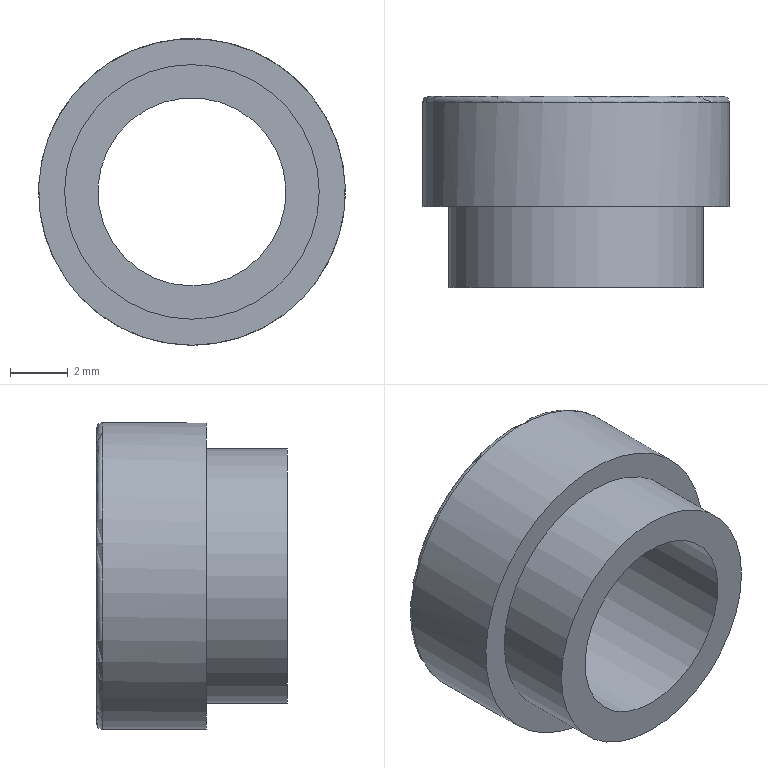Part | STEP file | 1 solid | 7 faces | box 10.6 x 6.6 x 10.6 mm | volume 286.348 mm3 | cylinder 3 | plane 3 | torus 1 | commonest cylinder face diameters 6.5 x1 8.8 x1 10.6 x1
STEP:
#1=CARTESIAN_POINT('',(0.,0.,0.));
#2=DIRECTION('',(0.,0.,1.));
#3=DIRECTION('',(1.,0.,0.));
#4=AXIS2_PLACEMENT_3D('',#1,#2,#3);
#5=CARTESIAN_POINT('',(0.,0.,-3.25));
#6=VERTEX_POINT('',#5);
#7=CARTESIAN_POINT('',(0.,0.,0.));
#8=DIRECTION('',(0.,1.,0.));
#9=DIRECTION('',(0.,0.,-1.));
#10=AXIS2_PLACEMENT_3D('',#7,#8,#9);
#11=CIRCLE('',#10,3.25);
#12=CARTESIAN_POINT('',(0.,6.93,0.));
#13=DIRECTION('',(0.,-1.,0.));
#14=DIRECTION('',(0.,0.,-1.));
#15=AXIS2_PLACEMENT_3D('',#12,#13,#14);
#16=CYLINDRICAL_SURFACE('',#15,3.25);
#17=CARTESIAN_POINT('',(6.283,6.93));
#18=DIRECTION('',(-1.,0.));
#19=VECTOR('',#18,1.);
#20=LINE('',#17,#19);
#21=(GEOMETRIC_REPRESENTATION_CONTEXT(2)PARAMETRIC_REPRESENTATION_CONTEXT()REPRESENTATION_CONTEXT('',''));
#22=DEFINITIONAL_REPRESENTATION('',(#20),#21);
#23=PCURVE('',#16,#22);
#24=CARTESIAN_POINT('',(0.,0.,0.));
#25=DIRECTION('',(0.,-1.,0.));
#26=DIRECTION('',(0.,0.,-1.));
#27=AXIS2_PLACEMENT_3D('',#24,#25,#26);
#28=PLANE('',#27);
#29=CARTESIAN_POINT('',(3.25,0.));
#30=CARTESIAN_POINT('',(3.25,-5.629));
#31=CARTESIAN_POINT('',(-1.625,-2.815));
#32=CARTESIAN_POINT('',(-6.5,0.));
#33=CARTESIAN_POINT('',(-1.625,2.815));
#34=CARTESIAN_POINT('',(3.25,5.629));
#35=CARTESIAN_POINT('',(3.25,0.));
#36=(BOUNDED_CURVE()B_SPLINE_CURVE(2,(#29,#30,#31,#32,#33,#34,#35),.UNSPECIFIED.,.T.,.F.)B_SPLINE_CURVE_WITH_KNOTS((1,2,2,2,2,1),(-2.094,0.,2.094,4.189,6.283,8.378),.UNSPECIFIED.)CURVE()GEOMETRIC_REPRESENTATION_ITEM()RATIONAL_B_SPLINE_CURVE((1.,0.5,1.,0.5,1.,0.5,1.))REPRESENTATION_ITEM(''));
#37=(GEOMETRIC_REPRESENTATION_CONTEXT(2)PARAMETRIC_REPRESENTATION_CONTEXT()REPRESENTATION_CONTEXT('',''));
#38=DEFINITIONAL_REPRESENTATION('',(#36),#37);
#39=PCURVE('',#28,#38);
#40=SURFACE_CURVE('',#11,(#23,#39),.PCURVE_S1.);
#41=EDGE_CURVE('',#6,#6,#40,.T.);
#42=ORIENTED_EDGE('',*,*,#41,.T.);
#43=CARTESIAN_POINT('',(0.,6.6,-3.25));
#44=VERTEX_POINT('',#43);
#45=CARTESIAN_POINT('',(0.,6.6,-3.25));
#46=CARTESIAN_POINT('',(0.,0.,-3.25));
#47=B_SPLINE_CURVE_WITH_KNOTS('',1,(#45,#46),.UNSPECIFIED.,.F.,.F.,(2,2),(0.33,6.93),.PIECEWISE_BEZIER_KNOTS.);
#48=CARTESIAN_POINT('',(0.,0.));
#49=DIRECTION('',(0.,1.));
#50=VECTOR('',#49,1.);
#51=LINE('',#48,#50);
#52=(GEOMETRIC_REPRESENTATION_CONTEXT(2)PARAMETRIC_REPRESENTATION_CONTEXT()REPRESENTATION_CONTEXT('',''));
#53=DEFINITIONAL_REPRESENTATION('',(#51),#52);
#54=PCURVE('',#16,#53);
#55=CARTESIAN_POINT('',(6.283,0.));
#56=DIRECTION('',(0.,1.));
#57=VECTOR('',#56,1.);
#58=LINE('',#55,#57);
#59=(GEOMETRIC_REPRESENTATION_CONTEXT(2)PARAMETRIC_REPRESENTATION_CONTEXT()REPRESENTATION_CONTEXT('',''));
#60=DEFINITIONAL_REPRESENTATION('',(#58),#59);
#61=PCURVE('',#16,#60);
#62=SEAM_CURVE('',#47,(#54,#61),.PCURVE_S1.);
#63=EDGE_CURVE('',#44,#6,#62,.T.);
#64=ORIENTED_EDGE('',*,*,#63,.F.);
#65=CARTESIAN_POINT('',(0.,6.6,0.));
#66=DIRECTION('',(0.,-1.,0.));
#67=DIRECTION('',(0.,0.,-1.));
#68=AXIS2_PLACEMENT_3D('',#65,#66,#67);
#69=CIRCLE('',#68,3.25);
#70=CARTESIAN_POINT('',(0.,0.33));
#71=DIRECTION('',(1.,0.));
#72=VECTOR('',#71,1.);
#73=LINE('',#70,#72);
#74=(GEOMETRIC_REPRESENTATION_CONTEXT(2)PARAMETRIC_REPRESENTATION_CONTEXT()REPRESENTATION_CONTEXT('',''));
#75=DEFINITIONAL_REPRESENTATION('',(#73),#74);
#76=PCURVE('',#16,#75);
#77=CARTESIAN_POINT('',(0.,6.6,0.));
#78=DIRECTION('',(0.,-1.,0.));
#79=DIRECTION('',(0.,0.,-1.));
#80=AXIS2_PLACEMENT_3D('',#77,#78,#79);
#81=PLANE('',#80);
#82=CARTESIAN_POINT('',(0.,0.));
#83=DIRECTION('',(1.,0.));
#84=AXIS2_PLACEMENT_2D('',#82,#83);
#85=CIRCLE('',#84,3.25);
#86=(GEOMETRIC_REPRESENTATION_CONTEXT(2)PARAMETRIC_REPRESENTATION_CONTEXT()REPRESENTATION_CONTEXT('',''));
#87=DEFINITIONAL_REPRESENTATION('',(#85),#86);
#88=PCURVE('',#81,#87);
#89=SURFACE_CURVE('',#69,(#76,#88),.PCURVE_S1.);
#90=EDGE_CURVE('',#44,#44,#89,.T.);
#91=ORIENTED_EDGE('',*,*,#90,.T.);
#92=ORIENTED_EDGE('',*,*,#63,.T.);
#93=EDGE_LOOP('',(#42,#64,#91,#92));
#94=FACE_BOUND('',#93,.F.);
#95=ADVANCED_FACE('',(#94),#16,.F.);
#96=ORIENTED_EDGE('',*,*,#90,.T.);
#97=EDGE_LOOP('',(#96));
#98=FACE_BOUND('',#97,.T.);
#99=CARTESIAN_POINT('',(5.098,6.6,-0.1551));
#100=VERTEX_POINT('',#99);
#101=CARTESIAN_POINT('',(5.1,6.6,0.000000697));
#102=VERTEX_POINT('',#101);
#103=CARTESIAN_POINT('',(5.098,6.6,-0.1551));
#104=CARTESIAN_POINT('',(5.099,6.6,-0.1034));
#105=CARTESIAN_POINT('',(5.1,6.6,-0.0517));
#106=CARTESIAN_POINT('',(5.1,6.6,0.000000697));
#107=B_SPLINE_CURVE_WITH_KNOTS('',3,(#103,#104,#105,#106),.UNSPECIFIED.,.F.,.F.,(4,4),(0.000002146,1.),.PIECEWISE_BEZIER_KNOTS.);
#108=CARTESIAN_POINT('',(0.1551,5.098));
#109=CARTESIAN_POINT('',(0.1034,5.099));
#110=CARTESIAN_POINT('',(0.0517,5.1));
#111=CARTESIAN_POINT('',(-0.000000697,5.1));
#112=B_SPLINE_CURVE_WITH_KNOTS('',3,(#108,#109,#110,#111),.UNSPECIFIED.,.F.,.F.,(4,4),(0.000002146,1.),.PIECEWISE_BEZIER_KNOTS.);
#113=(GEOMETRIC_REPRESENTATION_CONTEXT(2)PARAMETRIC_REPRESENTATION_CONTEXT()REPRESENTATION_CONTEXT('',''));
#114=DEFINITIONAL_REPRESENTATION('',(#112),#113);
#115=PCURVE('',#81,#114);
#116=CARTESIAN_POINT('',(0.,6.4,0.));
#117=DIRECTION('',(0.,-1.,0.));
#118=DIRECTION('',(1.,0.,0.));
#119=AXIS2_PLACEMENT_3D('',#116,#117,#118);
#120=TOROIDAL_SURFACE('',#119,5.1,0.2);
#121=CARTESIAN_POINT('',(6.253,4.712));
#122=CARTESIAN_POINT('',(6.283,4.712));
#123=B_SPLINE_CURVE_WITH_KNOTS('',1,(#121,#122),.UNSPECIFIED.,.F.,.F.,(2,2),(0.000002146,1.),.PIECEWISE_BEZIER_KNOTS.);
#124=(GEOMETRIC_REPRESENTATION_CONTEXT(2)PARAMETRIC_REPRESENTATION_CONTEXT()REPRESENTATION_CONTEXT('',''));
#125=DEFINITIONAL_REPRESENTATION('',(#123),#124);
#126=PCURVE('',#120,#125);
#127=SURFACE_CURVE('',#107,(#115,#126),.PCURVE_S1.);
#128=EDGE_CURVE('',#100,#102,#127,.T.);
#129=ORIENTED_EDGE('',*,*,#128,.F.);
#130=CARTESIAN_POINT('',(-5.1,6.6,-0.000000697));
#131=VERTEX_POINT('',#130);
#132=CARTESIAN_POINT('',(-5.1,6.6,-0.000000697));
#133=CARTESIAN_POINT('',(-5.1,6.6,-0.6611));
#134=CARTESIAN_POINT('',(-4.97,6.6,-1.322));
#135=CARTESIAN_POINT('',(-4.468,6.6,-2.546));
#136=CARTESIAN_POINT('',(-4.097,6.6,-3.108));
#137=CARTESIAN_POINT('',(-3.17,6.6,-4.05));
#138=CARTESIAN_POINT('',(-2.613,6.6,-4.429));
#139=CARTESIAN_POINT('',(-1.397,6.6,-4.949));
#140=CARTESIAN_POINT('',(-0.7386,6.6,-5.089));
#141=CARTESIAN_POINT('',(0.5835,6.6,-5.109));
#142=CARTESIAN_POINT('',(1.246,6.6,-4.989));
#143=CARTESIAN_POINT('',(2.477,6.6,-4.507));
#144=CARTESIAN_POINT('',(3.045,6.6,-4.144));
#145=CARTESIAN_POINT('',(4.001,6.6,-3.231));
#146=CARTESIAN_POINT('',(4.389,6.6,-2.68));
#147=CARTESIAN_POINT('',(4.927,6.6,-1.473));
#148=CARTESIAN_POINT('',(5.078,6.6,-0.8159));
#149=CARTESIAN_POINT('',(5.098,6.6,-0.1551));
#150=B_SPLINE_CURVE_WITH_KNOTS('',3,(#132,#133,#134,#135,#136,#137,#138,#139,#140,#141,#142,#143,#144,#145,#146,#147,#148,#149),.UNSPECIFIED.,.F.,.F.,(4,2,2,2,2,2,2,2,4),(0.000000044,0.125,0.25,0.375,0.5,0.625,0.75,0.875,1.),.UNSPECIFIED.);
#151=CARTESIAN_POINT('',(0.000000697,-5.1));
#152=CARTESIAN_POINT('',(0.6611,-5.1));
#153=CARTESIAN_POINT('',(1.322,-4.97));
#154=CARTESIAN_POINT('',(2.546,-4.468));
#155=CARTESIAN_POINT('',(3.108,-4.097));
#156=CARTESIAN_POINT('',(4.05,-3.17));
#157=CARTESIAN_POINT('',(4.429,-2.613));
#158=CARTESIAN_POINT('',(4.949,-1.397));
#159=CARTESIAN_POINT('',(5.089,-0.7386));
#160=CARTESIAN_POINT('',(5.109,0.5835));
#161=CARTESIAN_POINT('',(4.989,1.246));
#162=CARTESIAN_POINT('',(4.507,2.477));
#163=CARTESIAN_POINT('',(4.144,3.045));
#164=CARTESIAN_POINT('',(3.231,4.001));
#165=CARTESIAN_POINT('',(2.68,4.389));
#166=CARTESIAN_POINT('',(1.473,4.927));
#167=CARTESIAN_POINT('',(0.8159,5.078));
#168=CARTESIAN_POINT('',(0.1551,5.098));
#169=B_SPLINE_CURVE_WITH_KNOTS('',3,(#151,#152,#153,#154,#155,#156,#157,#158,#159,#160,#161,#162,#163,#164,#165,#166,#167,#168),.UNSPECIFIED.,.F.,.F.,(4,2,2,2,2,2,2,2,4),(0.000000044,0.125,0.25,0.375,0.5,0.625,0.75,0.875,1.),.UNSPECIFIED.);
#170=(GEOMETRIC_REPRESENTATION_CONTEXT(2)PARAMETRIC_REPRESENTATION_CONTEXT()REPRESENTATION_CONTEXT('',''));
#171=DEFINITIONAL_REPRESENTATION('',(#169),#170);
#172=PCURVE('',#81,#171);
#173=CARTESIAN_POINT('',(3.142,4.712));
#174=CARTESIAN_POINT('',(3.165,4.712));
#175=CARTESIAN_POINT('',(3.212,4.712));
#176=CARTESIAN_POINT('',(3.283,4.711));
#177=CARTESIAN_POINT('',(3.354,4.711));
#178=CARTESIAN_POINT('',(3.424,4.711));
#179=CARTESIAN_POINT('',(3.495,4.712));
#180=CARTESIAN_POINT('',(3.566,4.712));
#181=CARTESIAN_POINT('',(3.637,4.711));
#182=CARTESIAN_POINT('',(3.707,4.711));
#183=CARTESIAN_POINT('',(3.778,4.711));
#184=CARTESIAN_POINT('',(3.849,4.712));
#185=CARTESIAN_POINT('',(3.919,4.713));
#186=CARTESIAN_POINT('',(3.99,4.712));
#187=CARTESIAN_POINT('',(4.061,4.711));
#188=CARTESIAN_POINT('',(4.132,4.711));
#189=CARTESIAN_POINT('',(4.202,4.711));
#190=CARTESIAN_POINT('',(4.273,4.712));
#191=CARTESIAN_POINT('',(4.344,4.712));
#192=CARTESIAN_POINT('',(4.414,4.711));
#193=CARTESIAN_POINT('',(4.485,4.711));
#194=CARTESIAN_POINT('',(4.556,4.711));
#195=CARTESIAN_POINT('',(4.626,4.712));
#196=CARTESIAN_POINT('',(4.697,4.713));
#197=CARTESIAN_POINT('',(4.768,4.712));
#198=CARTESIAN_POINT('',(4.839,4.711));
#199=CARTESIAN_POINT('',(4.909,4.711));
#200=CARTESIAN_POINT('',(4.98,4.711));
#201=CARTESIAN_POINT('',(5.051,4.712));
#202=CARTESIAN_POINT('',(5.121,4.712));
#203=CARTESIAN_POINT('',(5.192,4.711));
#204=CARTESIAN_POINT('',(5.263,4.711));
#205=CARTESIAN_POINT('',(5.334,4.711));
#206=CARTESIAN_POINT('',(5.404,4.712));
#207=CARTESIAN_POINT('',(5.475,4.713));
#208=CARTESIAN_POINT('',(5.546,4.712));
#209=CARTESIAN_POINT('',(5.616,4.711));
#210=CARTESIAN_POINT('',(5.687,4.711));
#211=CARTESIAN_POINT('',(5.758,4.711));
#212=CARTESIAN_POINT('',(5.829,4.712));
#213=CARTESIAN_POINT('',(5.899,4.712));
#214=CARTESIAN_POINT('',(5.97,4.711));
#215=CARTESIAN_POINT('',(6.041,4.711));
#216=CARTESIAN_POINT('',(6.111,4.711));
#217=CARTESIAN_POINT('',(6.182,4.712));
#218=CARTESIAN_POINT('',(6.229,4.712));
#219=CARTESIAN_POINT('',(6.253,4.712));
#220=B_SPLINE_CURVE_WITH_KNOTS('',3,(#173,#174,#175,#176,#177,#178,#179,#180,#181,#182,#183,#184,#185,#186,#187,#188,#189,#190,#191,#192,#193,#194,#195,#196,#197,#198,#199,#200,#201,#202,#203,#204,#205,#206,#207,#208,#209,#210,#211,#212,#213,#214,#215,#216,#217,#218,#219),.UNSPECIFIED.,.F.,.F.,(4,1,1,1,1,1,1,1,1,1,1,1,1,1,1,1,1,1,1,1,1,1,1,1,1,1,1,1,1,1,1,1,1,1,1,1,1,1,1,1,1,1,1,1,4),(0.000000044,0.02273,0.04545,0.06818,0.09091,0.1136,0.1364,0.1591,0.1818,0.2045,0.2273,0.25,0.2727,0.2955,0.3182,0.3409,0.3636,0.3864,0.4091,0.4318,0.4545,0.4773,0.5,0.5227,0.5455,0.5682,0.5909,0.6136,0.6364,0.6591,0.6818,0.7045,0.7273,0.75,0.7727,0.7955,0.8182,0.8409,0.8636,0.8864,0.9091,0.9318,0.9545,0.9773,1.),.QUASI_UNIFORM_KNOTS.);
#221=(GEOMETRIC_REPRESENTATION_CONTEXT(2)PARAMETRIC_REPRESENTATION_CONTEXT()REPRESENTATION_CONTEXT('',''));
#222=DEFINITIONAL_REPRESENTATION('',(#220),#221);
#223=PCURVE('',#120,#222);
#224=SURFACE_CURVE('',#150,(#172,#223),.PCURVE_S1.);
#225=EDGE_CURVE('',#131,#100,#224,.T.);
#226=ORIENTED_EDGE('',*,*,#225,.F.);
#227=CARTESIAN_POINT('',(-5.098,6.6,0.1551));
#228=VERTEX_POINT('',#227);
#229=CARTESIAN_POINT('',(-5.098,6.6,0.1551));
#230=CARTESIAN_POINT('',(-5.099,6.6,0.1034));
#231=CARTESIAN_POINT('',(-5.1,6.6,0.0517));
#232=CARTESIAN_POINT('',(-5.1,6.6,-0.000000697));
#233=B_SPLINE_CURVE_WITH_KNOTS('',3,(#229,#230,#231,#232),.UNSPECIFIED.,.F.,.F.,(4,4),(0.000002196,1.),.PIECEWISE_BEZIER_KNOTS.);
#234=CARTESIAN_POINT('',(-0.1551,-5.098));
#235=CARTESIAN_POINT('',(-0.1034,-5.099));
#236=CARTESIAN_POINT('',(-0.0517,-5.1));
#237=CARTESIAN_POINT('',(0.000000697,-5.1));
#238=B_SPLINE_CURVE_WITH_KNOTS('',3,(#234,#235,#236,#237),.UNSPECIFIED.,.F.,.F.,(4,4),(0.000002196,1.),.PIECEWISE_BEZIER_KNOTS.);
#239=(GEOMETRIC_REPRESENTATION_CONTEXT(2)PARAMETRIC_REPRESENTATION_CONTEXT()REPRESENTATION_CONTEXT('',''));
#240=DEFINITIONAL_REPRESENTATION('',(#238),#239);
#241=PCURVE('',#81,#240);
#242=CARTESIAN_POINT('',(3.111,4.712));
#243=CARTESIAN_POINT('',(3.142,4.712));
#244=B_SPLINE_CURVE_WITH_KNOTS('',1,(#242,#243),.UNSPECIFIED.,.F.,.F.,(2,2),(0.000002196,1.),.PIECEWISE_BEZIER_KNOTS.);
#245=(GEOMETRIC_REPRESENTATION_CONTEXT(2)PARAMETRIC_REPRESENTATION_CONTEXT()REPRESENTATION_CONTEXT('',''));
#246=DEFINITIONAL_REPRESENTATION('',(#244),#245);
#247=PCURVE('',#120,#246);
#248=SURFACE_CURVE('',#233,(#241,#247),.PCURVE_S1.);
#249=EDGE_CURVE('',#228,#131,#248,.T.);
#250=ORIENTED_EDGE('',*,*,#249,.F.);
#251=CARTESIAN_POINT('',(5.1,6.6,0.000000697));
#252=CARTESIAN_POINT('',(5.1,6.6,0.6611));
#253=CARTESIAN_POINT('',(4.97,6.6,1.322));
#254=CARTESIAN_POINT('',(4.468,6.6,2.546));
#255=CARTESIAN_POINT('',(4.097,6.6,3.108));
#256=CARTESIAN_POINT('',(3.17,6.6,4.05));
#257=CARTESIAN_POINT('',(2.613,6.6,4.429));
#258=CARTESIAN_POINT('',(1.397,6.6,4.949));
#259=CARTESIAN_POINT('',(0.7386,6.6,5.089));
#260=CARTESIAN_POINT('',(-0.5835,6.6,5.109));
#261=CARTESIAN_POINT('',(-1.246,6.6,4.989));
#262=CARTESIAN_POINT('',(-2.477,6.6,4.507));
#263=CARTESIAN_POINT('',(-3.045,6.6,4.144));
#264=CARTESIAN_POINT('',(-4.001,6.6,3.231));
#265=CARTESIAN_POINT('',(-4.389,6.6,2.68));
#266=CARTESIAN_POINT('',(-4.927,6.6,1.473));
#267=CARTESIAN_POINT('',(-5.078,6.6,0.8159));
#268=CARTESIAN_POINT('',(-5.098,6.6,0.1551));
#269=B_SPLINE_CURVE_WITH_KNOTS('',3,(#251,#252,#253,#254,#255,#256,#257,#258,#259,#260,#261,#262,#263,#264,#265,#266,#267,#268),.UNSPECIFIED.,.F.,.F.,(4,2,2,2,2,2,2,2,4),(0.000000044,0.125,0.25,0.375,0.5,0.625,0.75,0.875,1.),.UNSPECIFIED.);
#270=CARTESIAN_POINT('',(-0.000000697,5.1));
#271=CARTESIAN_POINT('',(-0.6611,5.1));
#272=CARTESIAN_POINT('',(-1.322,4.97));
#273=CARTESIAN_POINT('',(-2.546,4.468));
#274=CARTESIAN_POINT('',(-3.108,4.097));
#275=CARTESIAN_POINT('',(-4.05,3.17));
#276=CARTESIAN_POINT('',(-4.429,2.613));
#277=CARTESIAN_POINT('',(-4.949,1.397));
#278=CARTESIAN_POINT('',(-5.089,0.7386));
#279=CARTESIAN_POINT('',(-5.109,-0.5835));
#280=CARTESIAN_POINT('',(-4.989,-1.246));
#281=CARTESIAN_POINT('',(-4.507,-2.477));
#282=CARTESIAN_POINT('',(-4.144,-3.045));
#283=CARTESIAN_POINT('',(-3.231,-4.001));
#284=CARTESIAN_POINT('',(-2.68,-4.389));
#285=CARTESIAN_POINT('',(-1.473,-4.927));
#286=CARTESIAN_POINT('',(-0.8159,-5.078));
#287=CARTESIAN_POINT('',(-0.1551,-5.098));
#288=B_SPLINE_CURVE_WITH_KNOTS('',3,(#270,#271,#272,#273,#274,#275,#276,#277,#278,#279,#280,#281,#282,#283,#284,#285,#286,#287),.UNSPECIFIED.,.F.,.F.,(4,2,2,2,2,2,2,2,4),(0.000000044,0.125,0.25,0.375,0.5,0.625,0.75,0.875,1.),.UNSPECIFIED.);
#289=(GEOMETRIC_REPRESENTATION_CONTEXT(2)PARAMETRIC_REPRESENTATION_CONTEXT()REPRESENTATION_CONTEXT('',''));
#290=DEFINITIONAL_REPRESENTATION('',(#288),#289);
#291=PCURVE('',#81,#290);
#292=CARTESIAN_POINT('',(0.000000137,4.712));
#293=CARTESIAN_POINT('',(0.02357,4.712));
#294=CARTESIAN_POINT('',(0.07071,4.712));
#295=CARTESIAN_POINT('',(0.1414,4.711));
#296=CARTESIAN_POINT('',(0.2121,4.711));
#297=CARTESIAN_POINT('',(0.2828,4.711));
#298=CARTESIAN_POINT('',(0.3535,4.712));
#299=CARTESIAN_POINT('',(0.4243,4.712));
#300=CARTESIAN_POINT('',(0.495,4.711));
#301=CARTESIAN_POINT('',(0.5657,4.711));
#302=CARTESIAN_POINT('',(0.6364,4.711));
#303=CARTESIAN_POINT('',(0.7071,4.712));
#304=CARTESIAN_POINT('',(0.7778,4.713));
#305=CARTESIAN_POINT('',(0.8485,4.712));
#306=CARTESIAN_POINT('',(0.9192,4.711));
#307=CARTESIAN_POINT('',(0.9899,4.711));
#308=CARTESIAN_POINT('',(1.061,4.711));
#309=CARTESIAN_POINT('',(1.131,4.712));
#310=CARTESIAN_POINT('',(1.202,4.712));
#311=CARTESIAN_POINT('',(1.273,4.711));
#312=CARTESIAN_POINT('',(1.343,4.711));
#313=CARTESIAN_POINT('',(1.414,4.711));
#314=CARTESIAN_POINT('',(1.485,4.712));
#315=CARTESIAN_POINT('',(1.556,4.713));
#316=CARTESIAN_POINT('',(1.626,4.712));
#317=CARTESIAN_POINT('',(1.697,4.711));
#318=CARTESIAN_POINT('',(1.768,4.711));
#319=CARTESIAN_POINT('',(1.838,4.711));
#320=CARTESIAN_POINT('',(1.909,4.712));
#321=CARTESIAN_POINT('',(1.98,4.712));
#322=CARTESIAN_POINT('',(2.051,4.711));
#323=CARTESIAN_POINT('',(2.121,4.711));
#324=CARTESIAN_POINT('',(2.192,4.711));
#325=CARTESIAN_POINT('',(2.263,4.712));
#326=CARTESIAN_POINT('',(2.333,4.713));
#327=CARTESIAN_POINT('',(2.404,4.712));
#328=CARTESIAN_POINT('',(2.475,4.711));
#329=CARTESIAN_POINT('',(2.546,4.711));
#330=CARTESIAN_POINT('',(2.616,4.711));
#331=CARTESIAN_POINT('',(2.687,4.712));
#332=CARTESIAN_POINT('',(2.758,4.712));
#333=CARTESIAN_POINT('',(2.828,4.711));
#334=CARTESIAN_POINT('',(2.899,4.711));
#335=CARTESIAN_POINT('',(2.97,4.711));
#336=CARTESIAN_POINT('',(3.04,4.712));
#337=CARTESIAN_POINT('',(3.088,4.712));
#338=CARTESIAN_POINT('',(3.111,4.712));
#339=B_SPLINE_CURVE_WITH_KNOTS('',3,(#292,#293,#294,#295,#296,#297,#298,#299,#300,#301,#302,#303,#304,#305,#306,#307,#308,#309,#310,#311,#312,#313,#314,#315,#316,#317,#318,#319,#320,#321,#322,#323,#324,#325,#326,#327,#328,#329,#330,#331,#332,#333,#334,#335,#336,#337,#338),.UNSPECIFIED.,.F.,.F.,(4,1,1,1,1,1,1,1,1,1,1,1,1,1,1,1,1,1,1,1,1,1,1,1,1,1,1,1,1,1,1,1,1,1,1,1,1,1,1,1,1,1,1,1,4),(0.000000044,0.02273,0.04545,0.06818,0.09091,0.1136,0.1364,0.1591,0.1818,0.2045,0.2273,0.25,0.2727,0.2955,0.3182,0.3409,0.3636,0.3864,0.4091,0.4318,0.4545,0.4773,0.5,0.5227,0.5455,0.5682,0.5909,0.6136,0.6364,0.6591,0.6818,0.7045,0.7273,0.75,0.7727,0.7955,0.8182,0.8409,0.8636,0.8864,0.9091,0.9318,0.9545,0.9773,1.),.QUASI_UNIFORM_KNOTS.);
#340=(GEOMETRIC_REPRESENTATION_CONTEXT(2)PARAMETRIC_REPRESENTATION_CONTEXT()REPRESENTATION_CONTEXT('',''));
#341=DEFINITIONAL_REPRESENTATION('',(#339),#340);
#342=PCURVE('',#120,#341);
#343=SURFACE_CURVE('',#269,(#291,#342),.PCURVE_S1.);
#344=EDGE_CURVE('',#102,#228,#343,.T.);
#345=ORIENTED_EDGE('',*,*,#344,.F.);
#346=EDGE_LOOP('',(#129,#226,#250,#345));
#347=FACE_BOUND('',#346,.T.);
#348=ADVANCED_FACE('',(#98,#347),#81,.F.);
#349=ORIENTED_EDGE('',*,*,#41,.T.);
#350=EDGE_LOOP('',(#349));
#351=FACE_BOUND('',#350,.T.);
#352=CARTESIAN_POINT('',(0.,0.,-4.4));
#353=VERTEX_POINT('',#352);
#354=CARTESIAN_POINT('',(0.,0.,0.));
#355=DIRECTION('',(0.,-1.,0.));
#356=DIRECTION('',(0.,0.,-1.));
#357=AXIS2_PLACEMENT_3D('',#354,#355,#356);
#358=CIRCLE('',#357,4.4);
#359=CARTESIAN_POINT('',(0.,0.));
#360=DIRECTION('',(1.,0.));
#361=AXIS2_PLACEMENT_2D('',#359,#360);
#362=CIRCLE('',#361,4.4);
#363=(GEOMETRIC_REPRESENTATION_CONTEXT(2)PARAMETRIC_REPRESENTATION_CONTEXT()REPRESENTATION_CONTEXT('',''));
#364=DEFINITIONAL_REPRESENTATION('',(#362),#363);
#365=PCURVE('',#28,#364);
#366=CARTESIAN_POINT('',(0.,6.93,0.));
#367=DIRECTION('',(0.,-1.,0.));
#368=DIRECTION('',(0.,0.,-1.));
#369=AXIS2_PLACEMENT_3D('',#366,#367,#368);
#370=CYLINDRICAL_SURFACE('',#369,4.4);
#371=CARTESIAN_POINT('',(0.,6.93));
#372=DIRECTION('',(1.,0.));
#373=VECTOR('',#372,1.);
#374=LINE('',#371,#373);
#375=(GEOMETRIC_REPRESENTATION_CONTEXT(2)PARAMETRIC_REPRESENTATION_CONTEXT()REPRESENTATION_CONTEXT('',''));
#376=DEFINITIONAL_REPRESENTATION('',(#374),#375);
#377=PCURVE('',#370,#376);
#378=SURFACE_CURVE('',#358,(#365,#377),.PCURVE_S1.);
#379=EDGE_CURVE('',#353,#353,#378,.T.);
#380=ORIENTED_EDGE('',*,*,#379,.T.);
#381=EDGE_LOOP('',(#380));
#382=FACE_BOUND('',#381,.T.);
#383=ADVANCED_FACE('',(#351,#382),#28,.T.);
#384=ORIENTED_EDGE('',*,*,#225,.T.);
#385=ORIENTED_EDGE('',*,*,#128,.T.);
#386=CARTESIAN_POINT('',(5.3,6.4,0.000000724));
#387=VERTEX_POINT('',#386);
#388=CARTESIAN_POINT('',(5.1,6.6,0.000000697));
#389=CARTESIAN_POINT('',(5.153,6.6,0.000000704));
#390=CARTESIAN_POINT('',(5.206,6.583,0.000000711));
#391=CARTESIAN_POINT('',(5.25,6.55,0.000000717));
#392=CARTESIAN_POINT('',(5.283,6.506,0.000000722));
#393=CARTESIAN_POINT('',(5.3,6.453,0.000000724));
#394=CARTESIAN_POINT('',(5.3,6.4,0.000000724));
#395=(BOUNDED_CURVE()B_SPLINE_CURVE(6,(#388,#389,#390,#391,#392,#393,#394),.UNSPECIFIED.,.F.,.F.)B_SPLINE_CURVE_WITH_KNOTS((7,7),(4.712,6.283),.PIECEWISE_BEZIER_KNOTS.)CURVE()GEOMETRIC_REPRESENTATION_ITEM()RATIONAL_B_SPLINE_CURVE((1.031,1.01,0.9979,0.994,0.9979,1.01,1.031))REPRESENTATION_ITEM(''));
#396=CARTESIAN_POINT('',(6.283,0.));
#397=DIRECTION('',(0.,1.));
#398=VECTOR('',#397,1.);
#399=LINE('',#396,#398);
#400=(GEOMETRIC_REPRESENTATION_CONTEXT(2)PARAMETRIC_REPRESENTATION_CONTEXT()REPRESENTATION_CONTEXT('',''));
#401=DEFINITIONAL_REPRESENTATION('',(#399),#400);
#402=PCURVE('',#120,#401);
#403=CARTESIAN_POINT('',(0.000000137,0.));
#404=DIRECTION('',(0.,1.));
#405=VECTOR('',#404,1.);
#406=LINE('',#403,#405);
#407=(GEOMETRIC_REPRESENTATION_CONTEXT(2)PARAMETRIC_REPRESENTATION_CONTEXT()REPRESENTATION_CONTEXT('',''));
#408=DEFINITIONAL_REPRESENTATION('',(#406),#407);
#409=PCURVE('',#120,#408);
#410=SEAM_CURVE('',#395,(#402,#409),.PCURVE_S1.);
#411=EDGE_CURVE('',#102,#387,#410,.T.);
#412=ORIENTED_EDGE('',*,*,#411,.T.);
#413=CARTESIAN_POINT('',(5.298,6.4,-0.1612));
#414=VERTEX_POINT('',#413);
#415=CARTESIAN_POINT('',(0.,6.4,0.));
#416=DIRECTION('',(0.,1.,0.));
#417=DIRECTION('',(0.9995,0.,-0.03041));
#418=AXIS2_PLACEMENT_3D('',#415,#416,#417);
#419=CIRCLE('',#418,5.3);
#420=CARTESIAN_POINT('',(12.536,6.283));
#421=DIRECTION('',(-1.,0.));
#422=VECTOR('',#421,1.);
#423=LINE('',#420,#422);
#424=(GEOMETRIC_REPRESENTATION_CONTEXT(2)PARAMETRIC_REPRESENTATION_CONTEXT()REPRESENTATION_CONTEXT('',''));
#425=DEFINITIONAL_REPRESENTATION('',(#423),#424);
#426=PCURVE('',#120,#425);
#427=CARTESIAN_POINT('',(0.,6.93,0.));
#428=DIRECTION('',(0.,-1.,0.));
#429=DIRECTION('',(0.,0.,-1.));
#430=AXIS2_PLACEMENT_3D('',#427,#428,#429);
#431=CYLINDRICAL_SURFACE('',#430,5.3);
#432=CARTESIAN_POINT('',(7.824,0.53));
#433=DIRECTION('',(-1.,0.));
#434=VECTOR('',#433,1.);
#435=LINE('',#432,#434);
#436=(GEOMETRIC_REPRESENTATION_CONTEXT(2)PARAMETRIC_REPRESENTATION_CONTEXT()REPRESENTATION_CONTEXT('',''));
#437=DEFINITIONAL_REPRESENTATION('',(#435),#436);
#438=PCURVE('',#431,#437);
#439=SURFACE_CURVE('',#419,(#426,#438),.PCURVE_S1.);
#440=EDGE_CURVE('',#387,#414,#439,.T.);
#441=ORIENTED_EDGE('',*,*,#440,.T.);
#442=CARTESIAN_POINT('',(0.,6.4,-5.3));
#443=VERTEX_POINT('',#442);
#444=CARTESIAN_POINT('',(0.,6.4,0.));
#445=DIRECTION('',(0.,1.,0.));
#446=DIRECTION('',(0.9995,0.,-0.03041));
#447=AXIS2_PLACEMENT_3D('',#444,#445,#446);
#448=CIRCLE('',#447,5.3);
#449=CARTESIAN_POINT('',(6.253,6.283));
#450=DIRECTION('',(-1.,0.));
#451=VECTOR('',#450,1.);
#452=LINE('',#449,#451);
#453=(GEOMETRIC_REPRESENTATION_CONTEXT(2)PARAMETRIC_REPRESENTATION_CONTEXT()REPRESENTATION_CONTEXT('',''));
#454=DEFINITIONAL_REPRESENTATION('',(#452),#453);
#455=PCURVE('',#120,#454);
#456=CARTESIAN_POINT('',(1.54,0.53));
#457=DIRECTION('',(-1.,0.));
#458=VECTOR('',#457,1.);
#459=LINE('',#456,#458);
#460=(GEOMETRIC_REPRESENTATION_CONTEXT(2)PARAMETRIC_REPRESENTATION_CONTEXT()REPRESENTATION_CONTEXT('',''));
#461=DEFINITIONAL_REPRESENTATION('',(#459),#460);
#462=PCURVE('',#431,#461);
#463=SURFACE_CURVE('',#448,(#455,#462),.PCURVE_S1.);
#464=EDGE_CURVE('',#414,#443,#463,.T.);
#465=ORIENTED_EDGE('',*,*,#464,.T.);
#466=CARTESIAN_POINT('',(0.,6.4,0.));
#467=DIRECTION('',(0.,1.,0.));
#468=DIRECTION('',(0.9995,0.,-0.03041));
#469=AXIS2_PLACEMENT_3D('',#466,#467,#468);
#470=CIRCLE('',#469,5.3);
#471=CARTESIAN_POINT('',(6.253,6.283));
#472=DIRECTION('',(-1.,0.));
#473=VECTOR('',#472,1.);
#474=LINE('',#471,#473);
#475=(GEOMETRIC_REPRESENTATION_CONTEXT(2)PARAMETRIC_REPRESENTATION_CONTEXT()REPRESENTATION_CONTEXT('',''));
#476=DEFINITIONAL_REPRESENTATION('',(#474),#475);
#477=PCURVE('',#120,#476);
#478=CARTESIAN_POINT('',(7.824,0.53));
#479=DIRECTION('',(-1.,0.));
#480=VECTOR('',#479,1.);
#481=LINE('',#478,#480);
#482=(GEOMETRIC_REPRESENTATION_CONTEXT(2)PARAMETRIC_REPRESENTATION_CONTEXT()REPRESENTATION_CONTEXT('',''));
#483=DEFINITIONAL_REPRESENTATION('',(#481),#482);
#484=PCURVE('',#431,#483);
#485=SURFACE_CURVE('',#470,(#477,#484),.PCURVE_S1.);
#486=EDGE_CURVE('',#443,#387,#485,.T.);
#487=ORIENTED_EDGE('',*,*,#486,.T.);
#488=ORIENTED_EDGE('',*,*,#411,.F.);
#489=ORIENTED_EDGE('',*,*,#344,.T.);
#490=ORIENTED_EDGE('',*,*,#249,.T.);
#491=EDGE_LOOP('',(#384,#385,#412,#441,#465,#487,#488,#489,#490));
#492=FACE_BOUND('',#491,.T.);
#493=ADVANCED_FACE('',(#492),#120,.T.);
#494=CARTESIAN_POINT('',(0.,2.8,-4.4));
#495=VERTEX_POINT('',#494);
#496=CARTESIAN_POINT('',(0.,2.8,0.));
#497=DIRECTION('',(0.,-1.,0.));
#498=DIRECTION('',(0.,0.,-1.));
#499=AXIS2_PLACEMENT_3D('',#496,#497,#498);
#500=CIRCLE('',#499,4.4);
#501=CARTESIAN_POINT('',(0.,4.13));
#502=DIRECTION('',(1.,0.));
#503=VECTOR('',#502,1.);
#504=LINE('',#501,#503);
#505=(GEOMETRIC_REPRESENTATION_CONTEXT(2)PARAMETRIC_REPRESENTATION_CONTEXT()REPRESENTATION_CONTEXT('',''));
#506=DEFINITIONAL_REPRESENTATION('',(#504),#505);
#507=PCURVE('',#370,#506);
#508=CARTESIAN_POINT('',(0.,2.8,0.));
#509=DIRECTION('',(0.,-1.,0.));
#510=DIRECTION('',(0.,0.,-1.));
#511=AXIS2_PLACEMENT_3D('',#508,#509,#510);
#512=PLANE('',#511);
#513=CARTESIAN_POINT('',(0.,0.));
#514=DIRECTION('',(1.,0.));
#515=AXIS2_PLACEMENT_2D('',#513,#514);
#516=CIRCLE('',#515,4.4);
#517=(GEOMETRIC_REPRESENTATION_CONTEXT(2)PARAMETRIC_REPRESENTATION_CONTEXT()REPRESENTATION_CONTEXT('',''));
#518=DEFINITIONAL_REPRESENTATION('',(#516),#517);
#519=PCURVE('',#512,#518);
#520=SURFACE_CURVE('',#500,(#507,#519),.PCURVE_S1.);
#521=EDGE_CURVE('',#495,#495,#520,.T.);
#522=ORIENTED_EDGE('',*,*,#521,.T.);
#523=CARTESIAN_POINT('',(0.,2.8,-4.4));
#524=CARTESIAN_POINT('',(0.,0.,-4.4));
#525=B_SPLINE_CURVE_WITH_KNOTS('',1,(#523,#524),.UNSPECIFIED.,.F.,.F.,(2,2),(4.13,6.93),.PIECEWISE_BEZIER_KNOTS.);
#526=CARTESIAN_POINT('',(6.283,0.));
#527=DIRECTION('',(0.,1.));
#528=VECTOR('',#527,1.);
#529=LINE('',#526,#528);
#530=(GEOMETRIC_REPRESENTATION_CONTEXT(2)PARAMETRIC_REPRESENTATION_CONTEXT()REPRESENTATION_CONTEXT('',''));
#531=DEFINITIONAL_REPRESENTATION('',(#529),#530);
#532=PCURVE('',#370,#531);
#533=CARTESIAN_POINT('',(0.,0.));
#534=DIRECTION('',(0.,1.));
#535=VECTOR('',#534,1.);
#536=LINE('',#533,#535);
#537=(GEOMETRIC_REPRESENTATION_CONTEXT(2)PARAMETRIC_REPRESENTATION_CONTEXT()REPRESENTATION_CONTEXT('',''));
#538=DEFINITIONAL_REPRESENTATION('',(#536),#537);
#539=PCURVE('',#370,#538);
#540=SEAM_CURVE('',#525,(#532,#539),.PCURVE_S1.);
#541=EDGE_CURVE('',#495,#353,#540,.T.);
#542=ORIENTED_EDGE('',*,*,#541,.T.);
#543=ORIENTED_EDGE('',*,*,#379,.F.);
#544=ORIENTED_EDGE('',*,*,#541,.F.);
#545=EDGE_LOOP('',(#522,#542,#543,#544));
#546=FACE_BOUND('',#545,.T.);
#547=ADVANCED_FACE('',(#546),#370,.T.);
#548=ORIENTED_EDGE('',*,*,#486,.F.);
#549=CARTESIAN_POINT('',(0.,2.8,-5.3));
#550=VERTEX_POINT('',#549);
#551=CARTESIAN_POINT('',(0.,6.4,-5.3));
#552=CARTESIAN_POINT('',(0.,2.8,-5.3));
#553=B_SPLINE_CURVE_WITH_KNOTS('',1,(#551,#552),.UNSPECIFIED.,.F.,.F.,(2,2),(0.53,4.13),.PIECEWISE_BEZIER_KNOTS.);
#554=CARTESIAN_POINT('',(6.283,0.));
#555=DIRECTION('',(0.,1.));
#556=VECTOR('',#555,1.);
#557=LINE('',#554,#556);
#558=(GEOMETRIC_REPRESENTATION_CONTEXT(2)PARAMETRIC_REPRESENTATION_CONTEXT()REPRESENTATION_CONTEXT('',''));
#559=DEFINITIONAL_REPRESENTATION('',(#557),#558);
#560=PCURVE('',#431,#559);
#561=CARTESIAN_POINT('',(0.,0.));
#562=DIRECTION('',(0.,1.));
#563=VECTOR('',#562,1.);
#564=LINE('',#561,#563);
#565=(GEOMETRIC_REPRESENTATION_CONTEXT(2)PARAMETRIC_REPRESENTATION_CONTEXT()REPRESENTATION_CONTEXT('',''));
#566=DEFINITIONAL_REPRESENTATION('',(#564),#565);
#567=PCURVE('',#431,#566);
#568=SEAM_CURVE('',#553,(#560,#567),.PCURVE_S1.);
#569=EDGE_CURVE('',#443,#550,#568,.T.);
#570=ORIENTED_EDGE('',*,*,#569,.T.);
#571=CARTESIAN_POINT('',(0.,2.8,0.));
#572=DIRECTION('',(0.,1.,0.));
#573=DIRECTION('',(0.,0.,-1.));
#574=AXIS2_PLACEMENT_3D('',#571,#572,#573);
#575=CIRCLE('',#574,5.3);
#576=CARTESIAN_POINT('',(6.283,4.13));
#577=DIRECTION('',(-1.,0.));
#578=VECTOR('',#577,1.);
#579=LINE('',#576,#578);
#580=(GEOMETRIC_REPRESENTATION_CONTEXT(2)PARAMETRIC_REPRESENTATION_CONTEXT()REPRESENTATION_CONTEXT('',''));
#581=DEFINITIONAL_REPRESENTATION('',(#579),#580);
#582=PCURVE('',#431,#581);
#583=CARTESIAN_POINT('',(5.3,0.));
#584=CARTESIAN_POINT('',(5.3,-9.18));
#585=CARTESIAN_POINT('',(-2.65,-4.59));
#586=CARTESIAN_POINT('',(-10.6,0.));
#587=CARTESIAN_POINT('',(-2.65,4.59));
#588=CARTESIAN_POINT('',(5.3,9.18));
#589=CARTESIAN_POINT('',(5.3,0.));
#590=(BOUNDED_CURVE()B_SPLINE_CURVE(2,(#583,#584,#585,#586,#587,#588,#589),.UNSPECIFIED.,.T.,.F.)B_SPLINE_CURVE_WITH_KNOTS((1,2,2,2,2,1),(-2.094,0.,2.094,4.189,6.283,8.378),.UNSPECIFIED.)CURVE()GEOMETRIC_REPRESENTATION_ITEM()RATIONAL_B_SPLINE_CURVE((1.,0.5,1.,0.5,1.,0.5,1.))REPRESENTATION_ITEM(''));
#591=(GEOMETRIC_REPRESENTATION_CONTEXT(2)PARAMETRIC_REPRESENTATION_CONTEXT()REPRESENTATION_CONTEXT('',''));
#592=DEFINITIONAL_REPRESENTATION('',(#590),#591);
#593=PCURVE('',#512,#592);
#594=SURFACE_CURVE('',#575,(#582,#593),.PCURVE_S1.);
#595=EDGE_CURVE('',#550,#550,#594,.T.);
#596=ORIENTED_EDGE('',*,*,#595,.T.);
#597=ORIENTED_EDGE('',*,*,#569,.F.);
#598=ORIENTED_EDGE('',*,*,#464,.F.);
#599=ORIENTED_EDGE('',*,*,#440,.F.);
#600=EDGE_LOOP('',(#548,#570,#596,#597,#598,#599));
#601=FACE_BOUND('',#600,.T.);
#602=ADVANCED_FACE('',(#601),#431,.T.);
#603=ORIENTED_EDGE('',*,*,#521,.F.);
#604=EDGE_LOOP('',(#603));
#605=FACE_BOUND('',#604,.T.);
#606=ORIENTED_EDGE('',*,*,#595,.F.);
#607=EDGE_LOOP('',(#606));
#608=FACE_BOUND('',#607,.T.);
#609=ADVANCED_FACE('',(#605,#608),#512,.T.);
#610=CLOSED_SHELL('',(#95,#348,#383,#493,#547,#602,#609));
#611=MANIFOLD_SOLID_BREP('',#610);
#612=(LENGTH_UNIT()NAMED_UNIT(*)SI_UNIT(.MILLI.,.METRE.));
#613=UNCERTAINTY_MEASURE_WITH_UNIT(LENGTH_MEASURE(0.000005),#612,'','');
#614=(NAMED_UNIT(*)PLANE_ANGLE_UNIT()SI_UNIT($,.RADIAN.));
#615=(NAMED_UNIT(*)SI_UNIT($,.STERADIAN.)SOLID_ANGLE_UNIT());
#616=(GEOMETRIC_REPRESENTATION_CONTEXT(3)GLOBAL_UNCERTAINTY_ASSIGNED_CONTEXT((#613))GLOBAL_UNIT_ASSIGNED_CONTEXT((#612,#614,#615))REPRESENTATION_CONTEXT('',''));
#617=ADVANCED_BREP_SHAPE_REPRESENTATION('',(#4,#611),#616);